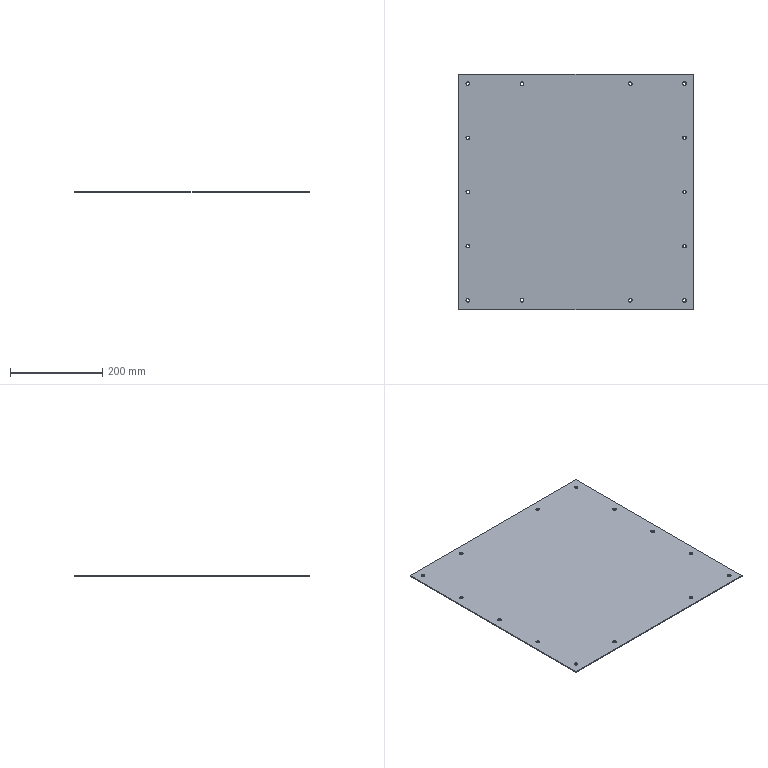Part | STEP file | Vibratory bowl feeder support plate | 1 solid | 66 faces | box 509.5 x 510 x 2 mm | volume 518611 mm3 | cylinder 32 | cone 28 | plane 6 | commonest cylinder face diameters 6.8 x28 1 x4